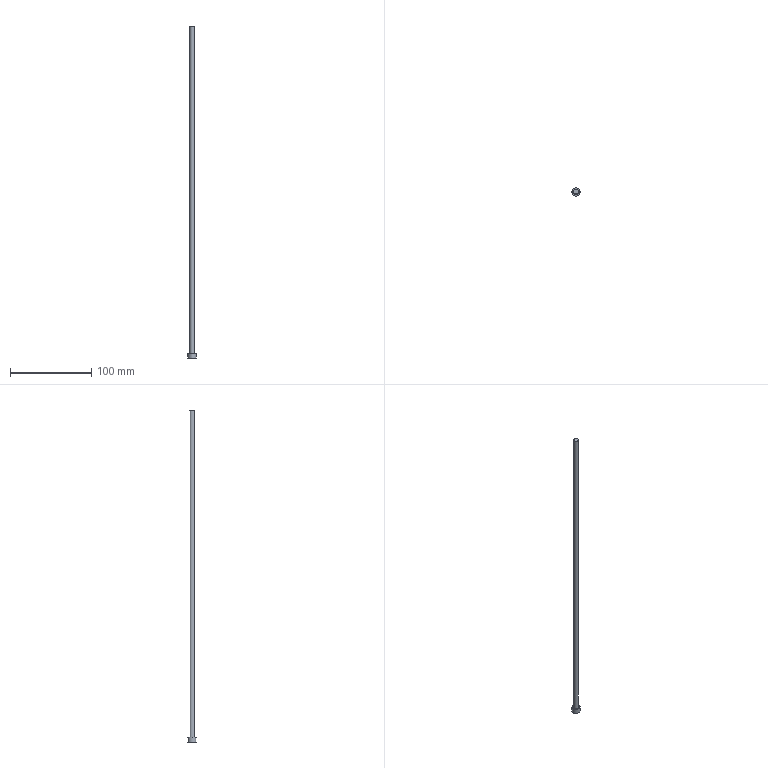Part | STEP file | solid 69 | 1 solid | 5 faces | box 10 x 10 x 408.49 mm | volume 11851 mm3 | plane 3 | cylinder 2 | commonest cylinder face diameters 6 x1 10 x1